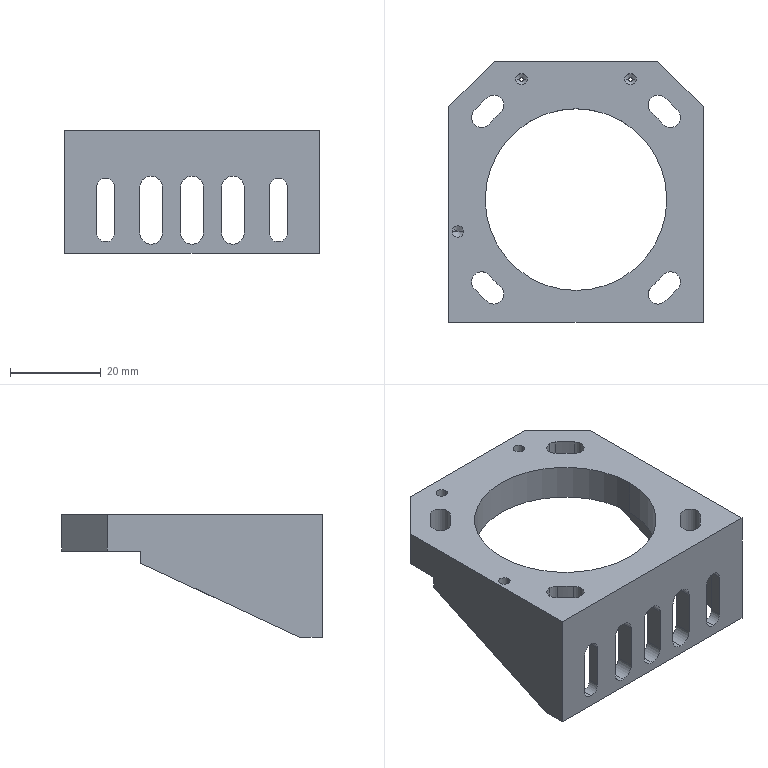NC program | NX | posted with a generic post | part box 56 x 57.4 x 27 mm
Lines 1 to 337 of 23725:
N10 G17 G21 G94 G90
(FLOOR_WALL_COPY , TOOL : D63)
N12 T02 M6
N14 G54
N16 G17 G0 G90 X-65.2 Y27.997 B0. C0. S2000 M3
N18 G43 Z30. H2
N20 Z5.9
N22 G94 G1 Z2.9 F1250.
N24 X-60.2
N26 X60.2
N28 Y-2.8
N30 X-60.2
N32 X-65.2
N34 Z5.9
N36 G0 Z30.
N38 Y27.997
N40 Z5.8
N42 G1 Z2.8
N44 X-60.2
N46 X60.2
N48 Y-2.8
N50 X-60.2
N52 X-65.2
N54 Z5.8
N56 G0 Z30.
N58 Y27.997
N60 Z5.7
N62 G1 Z2.7
N64 X-60.2
N66 X60.2
N68 Y-2.8
N70 X-60.2
N72 X-65.2
N74 Z5.7
N76 G0 Z30.
N78 Y27.997
N80 Z5.6
N82 G1 Z2.6
N84 X-60.2
N86 X60.2
N88 Y-2.8
N90 X-60.2
N92 X-65.2
N94 Z5.6
N96 G0 Z30.
N98 Y27.997
N100 Z5.5
N102 G1 Z2.5
N104 X-60.2
N106 X60.2
N108 Y-2.8
N110 X-60.2
N112 X-65.2
N114 Z5.5
N116 G0 Z30.
N118 Y27.997
N120 Z5.4
N122 G1 Z2.4
N124 X-60.2
N126 X60.2
N128 Y-2.8
N130 X-60.2
N132 X-65.2
N134 Z5.4
N136 G0 Z30.
N138 Y27.997
N140 Z5.3
N142 G1 Z2.3
N144 X-60.2
N146 X60.2
N148 Y-2.8
N150 X-60.2
N152 X-65.2
N154 Z5.3
N156 G0 Z30.
N158 Y27.997
N160 Z5.2
N162 G1 Z2.2
N164 X-60.2
N166 X60.2
N168 Y-2.8
N170 X-60.2
N172 X-65.2
N174 Z5.2
N176 G0 Z30.
N178 Y27.997
N180 Z5.1
N182 G1 Z2.1
N184 X-60.2
N186 X60.2
N188 Y-2.8
N190 X-60.2
N192 X-65.2
N194 Z5.1
N196 G0 Z30.
N198 Y27.997
N200 Z5.
N202 G1 Z2.
N204 X-60.2
N206 X60.2
N208 Y-2.8
N210 X-60.2
N212 X-65.2
N214 Z5.
N216 G0 Z30.
N218 Y27.997
N220 Z4.9
N222 G1 Z1.9
N224 X-60.2
N226 X60.2
N228 Y-2.8
N230 X-60.2
N232 X-65.2
N234 Z4.9
N236 G0 Z30.
N238 Y27.997
N240 Z4.8
N242 G1 Z1.8
N244 X-60.2
N246 X60.2
N248 Y-2.8
N250 X-60.2
N252 X-65.2
N254 Z4.8
N256 G0 Z30.
N258 Y27.997
N260 Z4.7
N262 G1 Z1.7
N264 X-60.2
N266 X60.2
N268 Y-2.8
N270 X-60.2
N272 X-65.2
N274 Z4.7
N276 G0 Z30.
N278 Y27.997
N280 Z4.6
N282 G1 Z1.6
N284 X-60.2
N286 X60.2
N288 Y-2.8
N290 X-60.2
N292 X-65.2
N294 Z4.6
N296 G0 Z30.
N298 Y27.997
N300 Z4.5
N302 G1 Z1.5
N304 X-60.2
N306 X60.2
N308 Y-2.8
N310 X-60.2
N312 X-65.2
N314 Z4.5
N316 G0 Z30.
N318 Y27.997
N320 Z4.4
N322 G1 Z1.4
N324 X-60.2
N326 X60.2
N328 Y-2.8
N330 X-60.2
N332 X-65.2
N334 Z4.4
N336 G0 Z30.
N338 Y27.997
N340 Z4.3
N342 G1 Z1.3
N344 X-60.2
N346 X60.2
N348 Y-2.8
N350 X-60.2
N352 X-65.2
N354 Z4.3
N356 G0 Z30.
N358 Y27.997
N360 Z4.2
N362 G1 Z1.2
N364 X-60.2
N366 X60.2
N368 Y-2.8
N370 X-60.2
N372 X-65.2
N374 Z4.2
N376 G0 Z30.
N378 Y27.997
N380 Z4.1
N382 G1 Z1.1
N384 X-60.2
N386 X60.2
N388 Y-2.8
N390 X-60.2
N392 X-65.2
N394 Z4.1
N396 G0 Z30.
N398 Y27.997
N400 Z4.
N402 G1 Z1.
N404 X-60.2
N406 X60.2
N408 Y-2.8
N410 X-60.2
N412 X-65.2
N414 Z4.
N416 G0 Z30.
N418 Y27.997
N420 Z3.9
N422 G1 Z0.9
N424 X-60.2
N426 X60.2
N428 Y-2.8
N430 X-60.2
N432 X-65.2
N434 Z3.9
N436 G0 Z30.
N438 Y27.997
N440 Z3.8
N442 G1 Z0.8
N444 X-60.2
N446 X60.2
N448 Y-2.8
N450 X-60.2
N452 X-65.2
N454 Z3.8
N456 G0 Z30.
N458 Y27.997
N460 Z3.7
N462 G1 Z0.7
N464 X-60.2
N466 X60.2
N468 Y-2.8
N470 X-60.2
N472 X-65.2
N474 Z3.7
N476 G0 Z30.
N478 Y27.997
N480 Z3.6
N482 G1 Z0.6
N484 X-60.2
N486 X60.2
N488 Y-2.8
N490 X-60.2
N492 X-65.2
N494 Z3.6
N496 G0 Z30.
N498 Y27.997
N500 Z3.5
N502 G1 Z0.5
N504 X-60.2
N506 X60.2
N508 Y-2.8
N510 X-60.2
N512 X-65.2
N514 Z3.5
N516 G0 Z30.
N518 Y27.997
N520 Z3.4
N522 G1 Z0.4
N524 X-60.2
N526 X60.2
N528 Y-2.8
N530 X-60.2
N532 X-65.2
N534 Z3.4
N536 G0 Z30.
N538 Y27.997
N540 Z3.3
N542 G1 Z0.3
N544 X-60.2
N546 X60.2
N548 Y-2.8
N550 X-60.2
N552 X-65.2
N554 Z3.3
N556 G0 Z30.
N558 Y27.997
N560 Z3.2
N562 G1 Z0.2
N564 X-60.2
N566 X60.2
N568 Y-2.8
N570 X-60.2
N572 X-65.2
N574 Z3.2
N576 G0 Z30.
N578 Y27.997
N580 Z3.1
N582 G1 Z0.1
N584 X-60.2
N586 X60.2
N588 Y-2.8
N590 X-60.2
N592 X-65.2
N594 Z3.1
N596 G0 Z30.
N598 M5
(FLOOR_WALL_COPY_COPY , TOOL : D10JING)
N600 T11 M6
N602 G54
N604 G17 G0 G90 X-38.7 Y27.997 B0. C0. S5000 M3
N606 G43 Z30. H11
N608 Z3.
N610 G94 G1 Z0. F1250.
N612 X-33.7
N614 X33.7
N616 Y23.27
N618 X-33.7
N620 Y18.543
N622 X33.7
N624 Y13.816
N626 X-33.7
N628 Y9.089
N630 X33.7
N632 Y4.362
N634 X-33.7
N636 Y-0.365
N638 X33.7
N640 Y-5.092
N642 X-33.7
N644 Y-9.819
N646 X33.7
N648 Y-14.546
N650 X-33.7
N652 Y-19.273
N654 X33.7
N656 Y-24.
N658 X-33.7
N660 X-38.7
N662 Z3.
N664 G0 Z30.
N666 M5